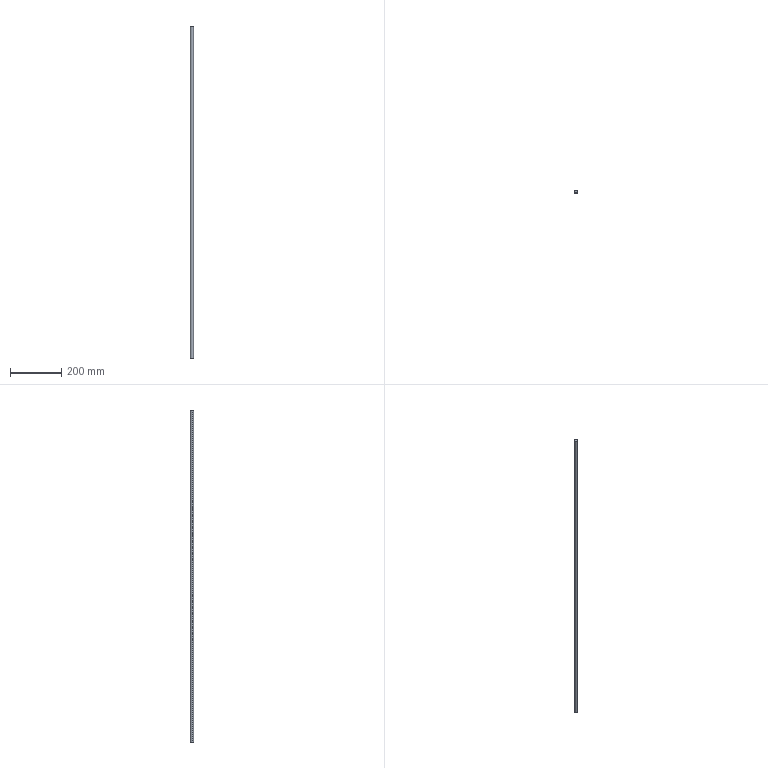Part | SolidWorks | features BaseBody 1 | 1 solid | 4 faces | box 12 x 12 x 1300 mm | volume 147027 mm3 | cylinder 2 | plane 2 | commonest cylinder face diameters 12 x2
STEP:
#1=CARTESIAN_POINT('',(-6.,0.,1300.));
#2=VERTEX_POINT('',#1);
#3=CARTESIAN_POINT('',(6.,0.,1300.));
#4=VERTEX_POINT('',#3);
#5=CARTESIAN_POINT('',(0.,0.,1300.));
#6=DIRECTION('',(0.,0.,-1.));
#7=DIRECTION('',(-1.,0.,0.));
#8=AXIS2_PLACEMENT_3D('',#5,#6,#7);
#9=CIRCLE('',#8,6.);
#10=EDGE_CURVE('',#2,#4,#9,.T.);
#11=ORIENTED_EDGE('',*,*,#10,.T.);
#12=CARTESIAN_POINT('',(6.,0.,0.));
#13=VERTEX_POINT('',#12);
#14=CARTESIAN_POINT('',(6.,0.,1300.));
#15=DIRECTION('',(0.,0.,-1.));
#16=VECTOR('',#15,1000.);
#17=LINE('',#14,#16);
#18=EDGE_CURVE('',#4,#13,#17,.T.);
#19=ORIENTED_EDGE('',*,*,#18,.T.);
#20=CARTESIAN_POINT('',(-6.,0.,0.));
#21=VERTEX_POINT('',#20);
#22=CARTESIAN_POINT('',(0.,0.,0.));
#23=DIRECTION('',(0.,0.,1.));
#24=DIRECTION('',(-1.,0.,0.));
#25=AXIS2_PLACEMENT_3D('',#22,#23,#24);
#26=CIRCLE('',#25,6.);
#27=EDGE_CURVE('',#13,#21,#26,.T.);
#28=ORIENTED_EDGE('',*,*,#27,.T.);
#29=CARTESIAN_POINT('',(-6.,0.,1300.));
#30=DIRECTION('',(0.,0.,-1.));
#31=VECTOR('',#30,1000.);
#32=LINE('',#29,#31);
#33=EDGE_CURVE('',#2,#21,#32,.T.);
#34=ORIENTED_EDGE('',*,*,#33,.F.);
#35=EDGE_LOOP('',(#11,#19,#28,#34));
#36=FACE_OUTER_BOUND('',#35,.T.);
#37=CARTESIAN_POINT('',(0.,0.,1300.));
#38=DIRECTION('',(0.,0.,-1.));
#39=DIRECTION('',(-1.,0.,0.));
#40=AXIS2_PLACEMENT_3D('',#37,#38,#39);
#41=CYLINDRICAL_SURFACE('',#40,6.);
#42=ADVANCED_FACE('',(#36),#41,.T.);
#43=ORIENTED_EDGE('',*,*,#18,.F.);
#44=CARTESIAN_POINT('',(0.,0.,1300.));
#45=DIRECTION('',(0.,0.,-1.));
#46=DIRECTION('',(-1.,0.,0.));
#47=AXIS2_PLACEMENT_3D('',#44,#45,#46);
#48=CIRCLE('',#47,6.);
#49=EDGE_CURVE('',#4,#2,#48,.T.);
#50=ORIENTED_EDGE('',*,*,#49,.T.);
#51=ORIENTED_EDGE('',*,*,#33,.T.);
#52=CARTESIAN_POINT('',(0.,0.,0.));
#53=DIRECTION('',(0.,0.,1.));
#54=DIRECTION('',(-1.,0.,0.));
#55=AXIS2_PLACEMENT_3D('',#52,#53,#54);
#56=CIRCLE('',#55,6.);
#57=EDGE_CURVE('',#21,#13,#56,.T.);
#58=ORIENTED_EDGE('',*,*,#57,.T.);
#59=EDGE_LOOP('',(#43,#50,#51,#58));
#60=FACE_OUTER_BOUND('',#59,.T.);
#61=CARTESIAN_POINT('',(0.,0.,1300.));
#62=DIRECTION('',(0.,0.,-1.));
#63=DIRECTION('',(-1.,0.,0.));
#64=AXIS2_PLACEMENT_3D('',#61,#62,#63);
#65=CYLINDRICAL_SURFACE('',#64,6.);
#66=ADVANCED_FACE('',(#60),#65,.T.);
#67=ORIENTED_EDGE('',*,*,#57,.F.);
#68=ORIENTED_EDGE('',*,*,#27,.F.);
#69=EDGE_LOOP('',(#67,#68));
#70=FACE_OUTER_BOUND('',#69,.T.);
#71=CARTESIAN_POINT('',(0.,0.,0.));
#72=DIRECTION('',(0.,0.,1.));
#73=DIRECTION('',(1.,0.,0.));
#74=AXIS2_PLACEMENT_3D('',#71,#72,#73);
#75=PLANE('',#74);
#76=ADVANCED_FACE('',(#70),#75,.F.);
#77=ORIENTED_EDGE('',*,*,#10,.F.);
#78=ORIENTED_EDGE('',*,*,#49,.F.);
#79=EDGE_LOOP('',(#77,#78));
#80=FACE_OUTER_BOUND('',#79,.T.);
#81=CARTESIAN_POINT('',(0.,0.,1300.));
#82=DIRECTION('',(0.,0.,1.));
#83=DIRECTION('',(1.,0.,0.));
#84=AXIS2_PLACEMENT_3D('',#81,#82,#83);
#85=PLANE('',#84);
#86=ADVANCED_FACE('',(#80),#85,.T.);
#87=CLOSED_SHELL('',(#42,#66,#76,#86));
#88=MANIFOLD_SOLID_BREP('',#87);
#89=CARTESIAN_POINT('',(0.,0.,0.));
#90=DIRECTION('',(0.,0.,1.));
#91=DIRECTION('',(1.,0.,0.));
#92=AXIS2_PLACEMENT_3D('',#89,#90,#91);
#93=(LENGTH_UNIT()NAMED_UNIT(*)SI_UNIT(.MILLI.,.METRE.));
#94=UNCERTAINTY_MEASURE_WITH_UNIT(LENGTH_MEASURE(0.00001),#93,'','');
#95=(NAMED_UNIT(*)PLANE_ANGLE_UNIT()SI_UNIT($,.RADIAN.));
#96=(NAMED_UNIT(*)SI_UNIT($,.STERADIAN.)SOLID_ANGLE_UNIT());
#97=(GEOMETRIC_REPRESENTATION_CONTEXT(3)GLOBAL_UNCERTAINTY_ASSIGNED_CONTEXT((#94))GLOBAL_UNIT_ASSIGNED_CONTEXT((#93,#95,#96))REPRESENTATION_CONTEXT('',''));
#98=ADVANCED_BREP_SHAPE_REPRESENTATION('',(#88,#92),#97);